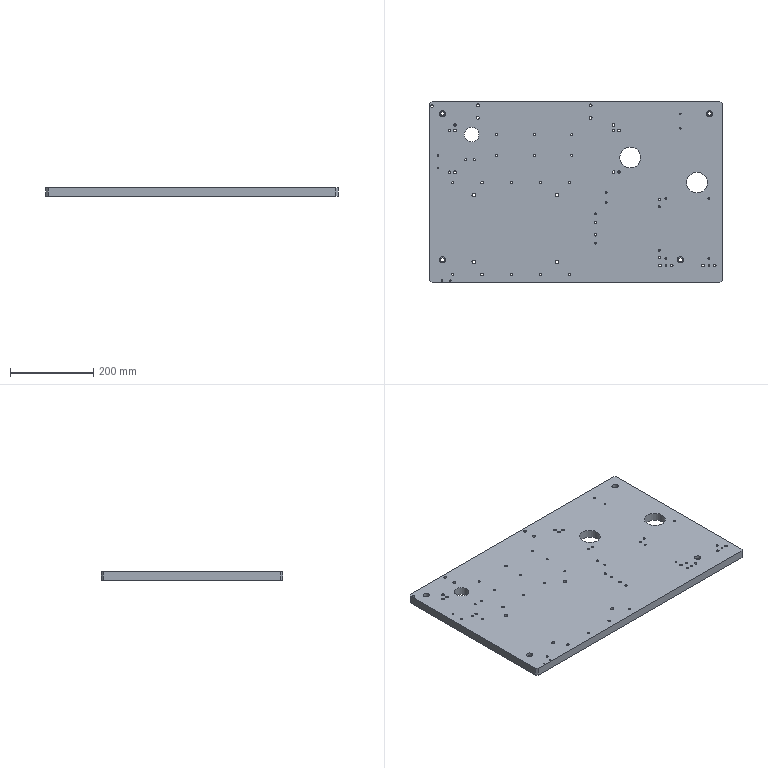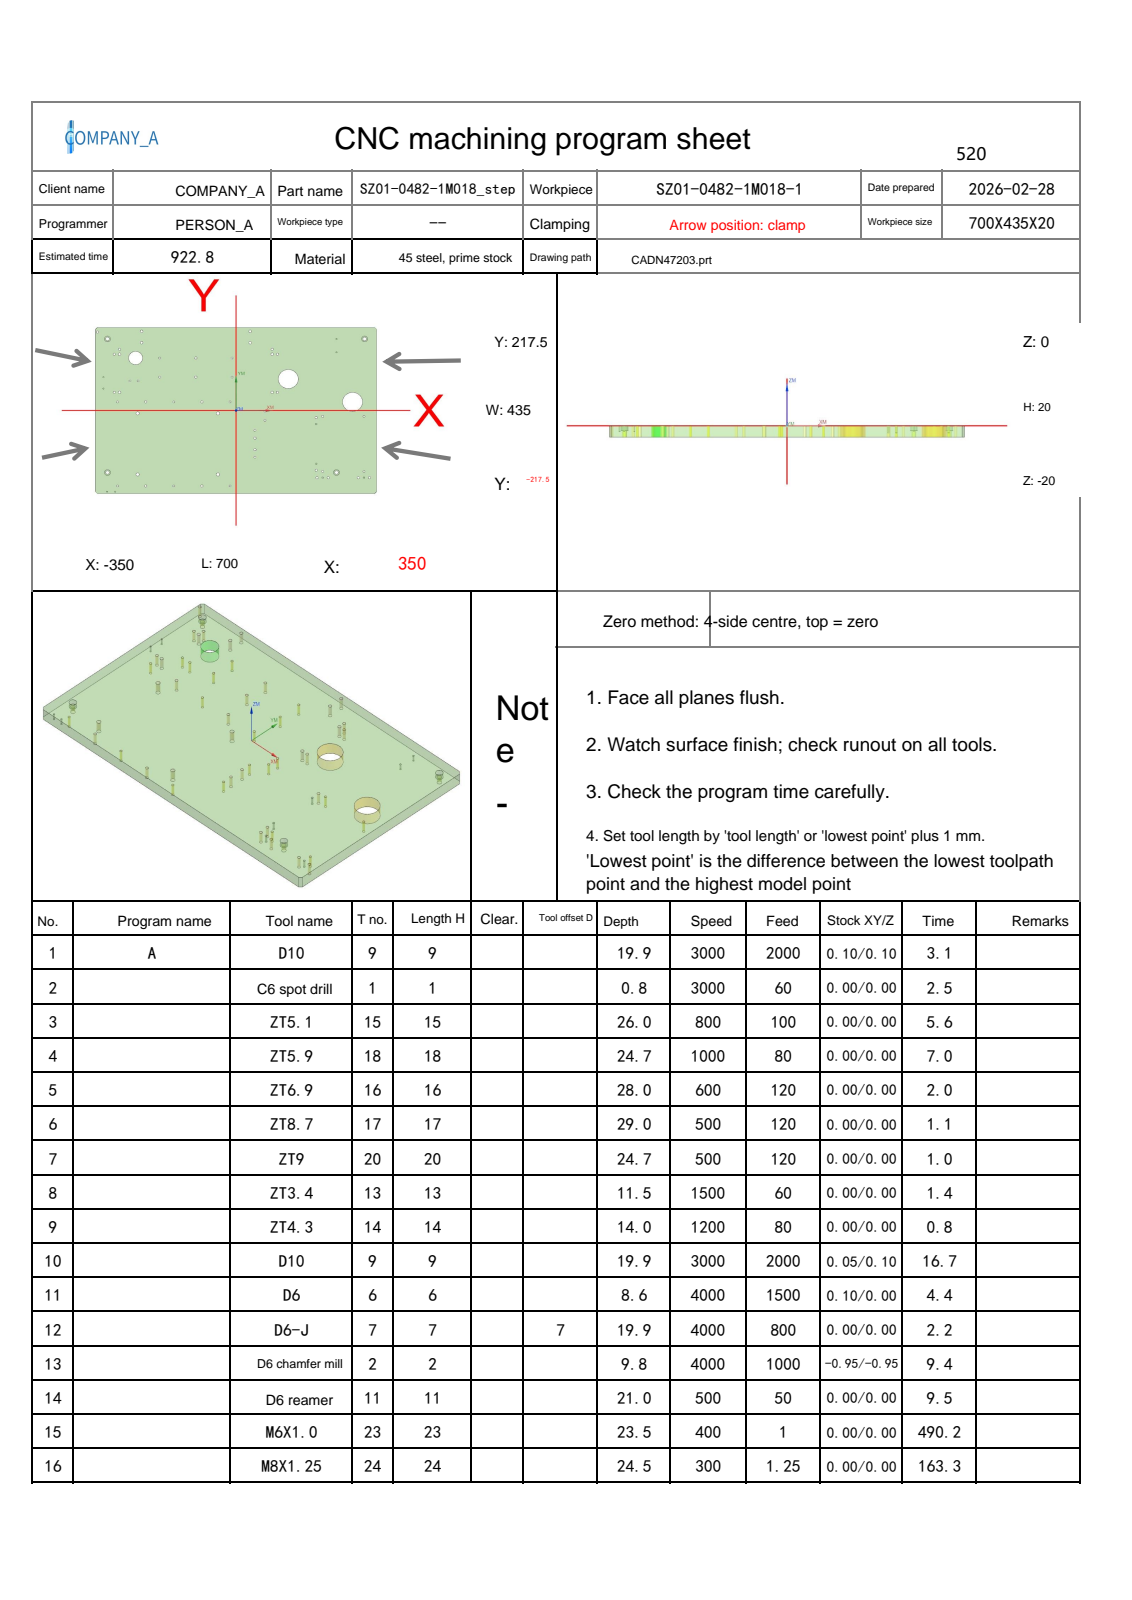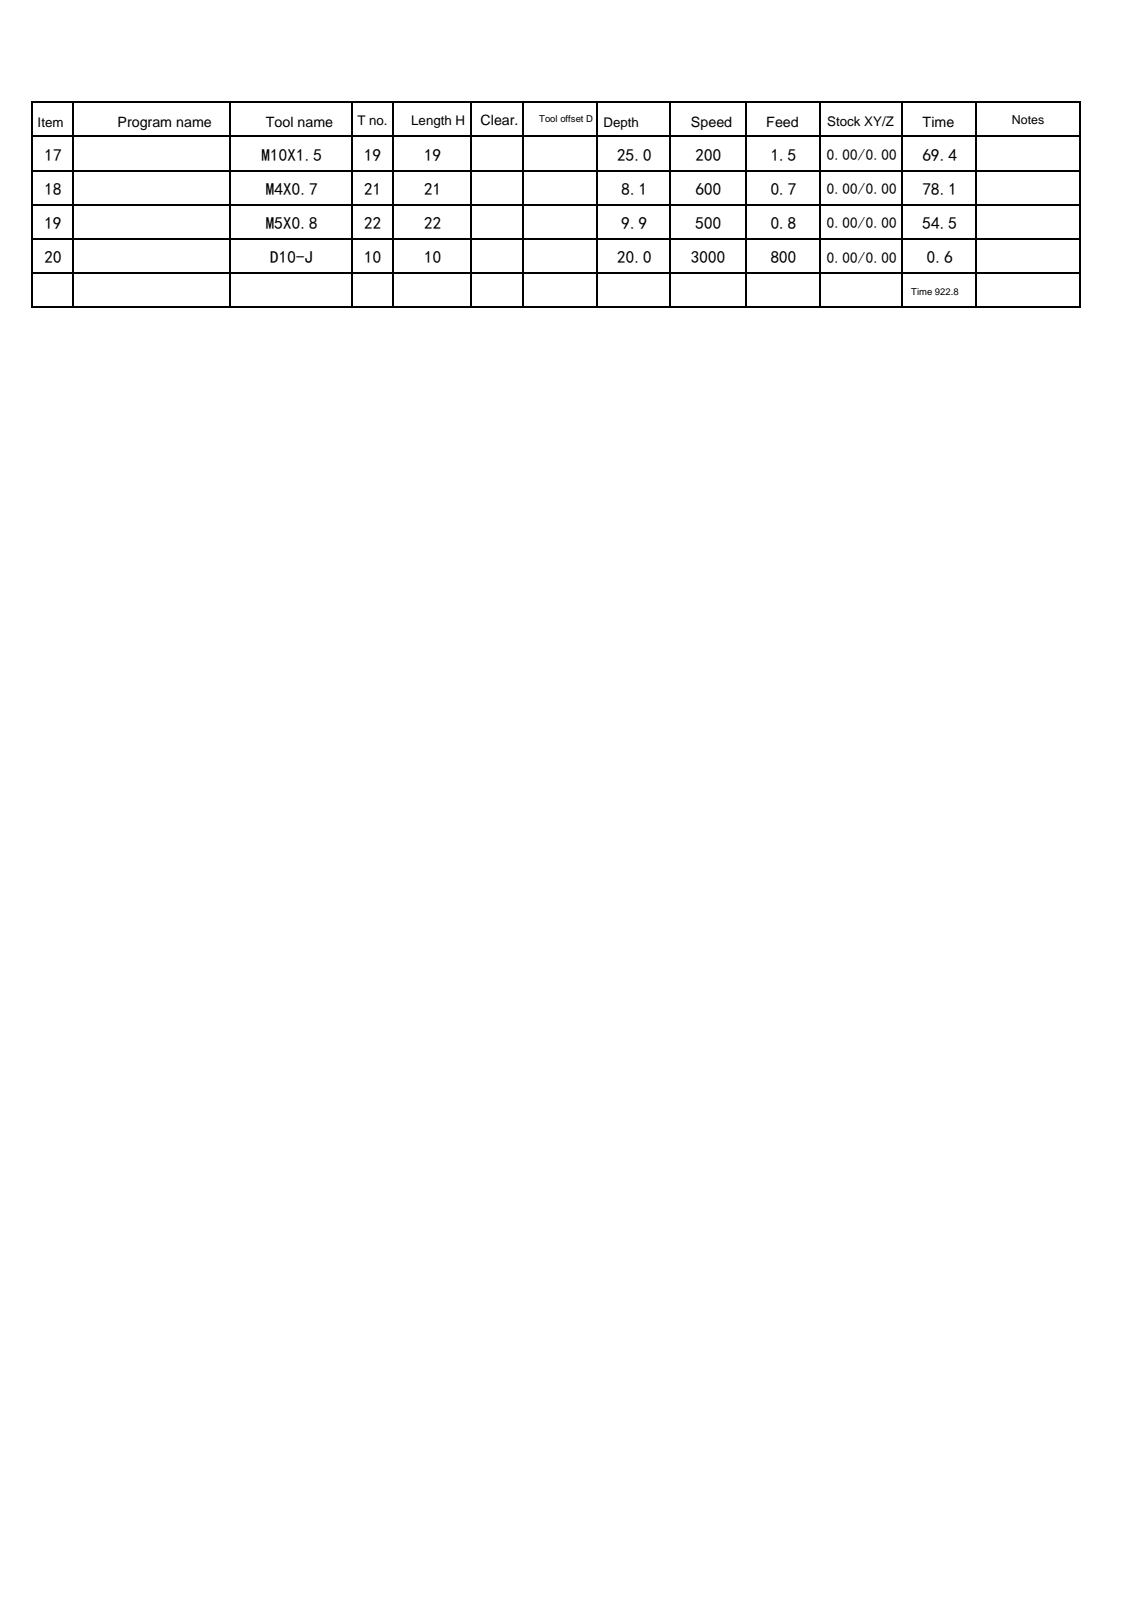NC program | NX | posted by the shop | part box 700 x 435 x 20 mm
Lines 2453 to 3078 of 5271:
N11 T06 M06
(D6  D=6. R=0. H=06 ce=0.10 di=0.00)
G00 G90 G54 X250. Y-162.5 M03 S4000
G43 H06 Z50.
M08
Z.5
G03 X251.1 Y-163.6 I1.1 J0.0 F1500.
X252.2 Y-162.5 I0.0 J1.1
X252.2 Y-162.5 Z.25 I-2.2 J0.0
X252.2 Y-162.5 Z0.0 I-2.2 J0.0
X252.2 Y-162.5 Z-.25 I-2.2 J0.0
X252.2 Y-162.5 Z-.5 I-2.2 J0.0
X252.2 Y-162.5 Z-.75 I-2.2 J0.0
X252.2 Y-162.5 Z-1. I-2.2 J0.0
X252.2 Y-162.5 Z-1.25 I-2.2 J0.0
X252.2 Y-162.5 Z-1.5 I-2.2 J0.0
X252.2 Y-162.5 Z-1.75 I-2.2 J0.0
X252.2 Y-162.5 Z-2. I-2.2 J0.0
X252.2 Y-162.5 Z-2.25 I-2.2 J0.0
X252.2 Y-162.5 Z-2.5 I-2.2 J0.0
X252.2 Y-162.5 Z-2.75 I-2.2 J0.0
X252.2 Y-162.5 Z-3. I-2.2 J0.0
X252.2 Y-162.5 Z-3.25 I-2.2 J0.0
X252.2 Y-162.5 Z-3.5 I-2.2 J0.0
X252.2 Y-162.5 Z-3.75 I-2.2 J0.0
X252.2 Y-162.5 Z-4. I-2.2 J0.0
X252.2 Y-162.5 Z-4.25 I-2.2 J0.0
X252.2 Y-162.5 Z-4.5 I-2.2 J0.0
X252.2 Y-162.5 Z-4.75 I-2.2 J0.0
X252.2 Y-162.5 Z-5. I-2.2 J0.0
X252.2 Y-162.5 Z-5.25 I-2.2 J0.0
X252.2 Y-162.5 Z-5.5 I-2.2 J0.0
X252.2 Y-162.5 Z-5.75 I-2.2 J0.0
X252.2 Y-162.5 Z-6. I-2.2 J0.0
X252.2 Y-162.5 Z-6.25 I-2.2 J0.0
X252.2 Y-162.5 Z-6.5 I-2.2 J0.0
X252.2 Y-162.5 Z-6.75 I-2.2 J0.0
X252.2 Y-162.5 Z-7. I-2.2 J0.0
X252.2 Y-162.5 Z-7.25 I-2.2 J0.0
X252.2 Y-162.5 Z-7.5 I-2.2 J0.0
X252.2 Y-162.5 Z-7.75 I-2.2 J0.0
X252.2 Y-162.5 Z-8. I-2.2 J0.0
X252.2 Y-162.5 Z-8.25 I-2.2 J0.0
X252.2 Y-162.5 Z-8.5 I-2.2 J0.0
X248.22 Y-161.207 Z-8.6 I-2.2 J0.0
X247.8 Y-162.5 I1.78 J-1.293
X250. Y-164.7 I2.2 J0.0
X252.2 Y-162.5 I0.0 J2.2
X250. Y-160.3 I-2.2 J0.0
X248.22 Y-161.207 I0.0 J-2.2
X248.01 Y-161.853 I.89 J-.647
X249.11 Y-162.953 I1.1 J0.0
X250. Y-162.5 I0.0 J1.1
G00 Z.5
G03 X252.2 Y-164.7 I2.2 J0.0
X254.4 Y-162.5 I0.0 J2.2
X254.4 Y-162.5 Z.25 I-4.4 J0.0
X254.4 Y-162.5 Z0.0 I-4.4 J0.0
X254.4 Y-162.5 Z-.25 I-4.4 J0.0
X254.4 Y-162.5 Z-.5 I-4.4 J0.0
X254.4 Y-162.5 Z-.75 I-4.4 J0.0
X254.4 Y-162.5 Z-1. I-4.4 J0.0
X254.4 Y-162.5 Z-1.25 I-4.4 J0.0
X254.4 Y-162.5 Z-1.5 I-4.4 J0.0
X254.4 Y-162.5 Z-1.75 I-4.4 J0.0
X254.4 Y-162.5 Z-2. I-4.4 J0.0
X254.4 Y-162.5 Z-2.25 I-4.4 J0.0
X254.4 Y-162.5 Z-2.5 I-4.4 J0.0
X254.4 Y-162.5 Z-2.75 I-4.4 J0.0
X254.4 Y-162.5 Z-3. I-4.4 J0.0
X254.4 Y-162.5 Z-3.25 I-4.4 J0.0
X254.4 Y-162.5 Z-3.5 I-4.4 J0.0
X254.4 Y-162.5 Z-3.75 I-4.4 J0.0
X254.4 Y-162.5 Z-4. I-4.4 J0.0
X254.4 Y-162.5 Z-4.25 I-4.4 J0.0
X254.4 Y-162.5 Z-4.5 I-4.4 J0.0
X254.4 Y-162.5 Z-4.75 I-4.4 J0.0
X254.4 Y-162.5 Z-5. I-4.4 J0.0
X254.4 Y-162.5 Z-5.25 I-4.4 J0.0
X254.4 Y-162.5 Z-5.5 I-4.4 J0.0
X254.4 Y-162.5 Z-5.75 I-4.4 J0.0
X254.4 Y-162.5 Z-6. I-4.4 J0.0
X254.4 Y-162.5 Z-6.25 I-4.4 J0.0
X254.4 Y-162.5 Z-6.5 I-4.4 J0.0
X254.4 Y-162.5 Z-6.75 I-4.4 J0.0
X254.4 Y-162.5 Z-7. I-4.4 J0.0
X254.4 Y-162.5 Z-7.25 I-4.4 J0.0
X254.4 Y-162.5 Z-7.5 I-4.4 J0.0
X254.4 Y-162.5 Z-7.75 I-4.4 J0.0
X254.4 Y-162.5 Z-8. I-4.4 J0.0
X254.4 Y-162.5 Z-8.25 I-4.4 J0.0
X254.4 Y-162.5 Z-8.5 I-4.4 J0.0
X246.44 Y-159.914 Z-8.6 I-4.4 J0.0
X245.6 Y-162.5 I3.56 J-2.586
X250. Y-166.9 I4.4 J0.0
X254.4 Y-162.5 I0.0 J4.4
X250. Y-158.1 I-4.4 J0.0
X246.44 Y-159.914 I0.0 J-4.4
X246.02 Y-161.207 I1.78 J-1.293
X248.22 Y-163.407 I2.2 J0.0
X250. Y-162.5 I0.0 J2.2
G00 Z50.
X320. Y187.5
Z.5
G03 X321.1 Y186.4 I1.1 J0.0
X322.2 Y187.5 I0.0 J1.1
X322.2 Y187.5 Z.25 I-2.2 J0.0
X322.2 Y187.5 Z0.0 I-2.2 J0.0
X322.2 Y187.5 Z-.25 I-2.2 J0.0
X322.2 Y187.5 Z-.5 I-2.2 J0.0
X322.2 Y187.5 Z-.75 I-2.2 J0.0
X322.2 Y187.5 Z-1. I-2.2 J0.0
X322.2 Y187.5 Z-1.25 I-2.2 J0.0
X322.2 Y187.5 Z-1.5 I-2.2 J0.0
X322.2 Y187.5 Z-1.75 I-2.2 J0.0
X322.2 Y187.5 Z-2. I-2.2 J0.0
X322.2 Y187.5 Z-2.25 I-2.2 J0.0
X322.2 Y187.5 Z-2.5 I-2.2 J0.0
X322.2 Y187.5 Z-2.75 I-2.2 J0.0
X322.2 Y187.5 Z-3. I-2.2 J0.0
X322.2 Y187.5 Z-3.25 I-2.2 J0.0
X322.2 Y187.5 Z-3.5 I-2.2 J0.0
X322.2 Y187.5 Z-3.75 I-2.2 J0.0
X322.2 Y187.5 Z-4. I-2.2 J0.0
X322.2 Y187.5 Z-4.25 I-2.2 J0.0
X322.2 Y187.5 Z-4.5 I-2.2 J0.0
X322.2 Y187.5 Z-4.75 I-2.2 J0.0
X322.2 Y187.5 Z-5. I-2.2 J0.0
X322.2 Y187.5 Z-5.25 I-2.2 J0.0
X322.2 Y187.5 Z-5.5 I-2.2 J0.0
X322.2 Y187.5 Z-5.75 I-2.2 J0.0
X322.2 Y187.5 Z-6. I-2.2 J0.0
X322.2 Y187.5 Z-6.25 I-2.2 J0.0
X322.2 Y187.5 Z-6.5 I-2.2 J0.0
X322.2 Y187.5 Z-6.75 I-2.2 J0.0
X322.2 Y187.5 Z-7. I-2.2 J0.0
X322.2 Y187.5 Z-7.25 I-2.2 J0.0
X322.2 Y187.5 Z-7.5 I-2.2 J0.0
X322.2 Y187.5 Z-7.75 I-2.2 J0.0
X322.2 Y187.5 Z-8. I-2.2 J0.0
X322.2 Y187.5 Z-8.25 I-2.2 J0.0
X322.2 Y187.5 Z-8.5 I-2.2 J0.0
X318.22 Y188.793 Z-8.6 I-2.2 J0.0
X317.8 Y187.5 I1.78 J-1.293
X320. Y185.3 I2.2 J0.0
X322.2 Y187.5 I0.0 J2.2
X320. Y189.7 I-2.2 J0.0
X318.22 Y188.793 I0.0 J-2.2
X318.01 Y188.147 I.89 J-.647
X319.11 Y187.047 I1.1 J0.0
X320. Y187.5 I0.0 J1.1
G00 Z.5
G03 X322.2 Y185.3 I2.2 J0.0
X324.4 Y187.5 I0.0 J2.2
X324.4 Y187.5 Z.25 I-4.4 J0.0
X324.4 Y187.5 Z0.0 I-4.4 J0.0
X324.4 Y187.5 Z-.25 I-4.4 J0.0
X324.4 Y187.5 Z-.5 I-4.4 J0.0
X324.4 Y187.5 Z-.75 I-4.4 J0.0
X324.4 Y187.5 Z-1. I-4.4 J0.0
X324.4 Y187.5 Z-1.25 I-4.4 J0.0
X324.4 Y187.5 Z-1.5 I-4.4 J0.0
X324.4 Y187.5 Z-1.75 I-4.4 J0.0
X324.4 Y187.5 Z-2. I-4.4 J0.0
X324.4 Y187.5 Z-2.25 I-4.4 J0.0
X324.4 Y187.5 Z-2.5 I-4.4 J0.0
X324.4 Y187.5 Z-2.75 I-4.4 J0.0
X324.4 Y187.5 Z-3. I-4.4 J0.0
X324.4 Y187.5 Z-3.25 I-4.4 J0.0
X324.4 Y187.5 Z-3.5 I-4.4 J0.0
X324.4 Y187.5 Z-3.75 I-4.4 J0.0
X324.4 Y187.5 Z-4. I-4.4 J0.0
X324.4 Y187.5 Z-4.25 I-4.4 J0.0
X324.4 Y187.5 Z-4.5 I-4.4 J0.0
X324.4 Y187.5 Z-4.75 I-4.4 J0.0
X324.4 Y187.5 Z-5. I-4.4 J0.0
X324.4 Y187.5 Z-5.25 I-4.4 J0.0
X324.4 Y187.5 Z-5.5 I-4.4 J0.0
X324.4 Y187.5 Z-5.75 I-4.4 J0.0
X324.4 Y187.5 Z-6. I-4.4 J0.0
X324.4 Y187.5 Z-6.25 I-4.4 J0.0
X324.4 Y187.5 Z-6.5 I-4.4 J0.0
X324.4 Y187.5 Z-6.75 I-4.4 J0.0
X324.4 Y187.5 Z-7. I-4.4 J0.0
X324.4 Y187.5 Z-7.25 I-4.4 J0.0
X324.4 Y187.5 Z-7.5 I-4.4 J0.0
X324.4 Y187.5 Z-7.75 I-4.4 J0.0
X324.4 Y187.5 Z-8. I-4.4 J0.0
X324.4 Y187.5 Z-8.25 I-4.4 J0.0
X324.4 Y187.5 Z-8.5 I-4.4 J0.0
X316.44 Y190.086 Z-8.6 I-4.4 J0.0
X315.6 Y187.5 I3.56 J-2.586
X320. Y183.1 I4.4 J0.0
X324.4 Y187.5 I0.0 J4.4
X320. Y191.9 I-4.4 J0.0
X316.44 Y190.086 I0.0 J-4.4
X316.02 Y188.793 I1.78 J-1.293
X318.22 Y186.593 I2.2 J0.0
X320. Y187.5 I0.0 J2.2
G00 Z50.
X-320.
Z.5
G03 X-318.9 Y186.4 I1.1 J0.0
X-317.8 Y187.5 I0.0 J1.1
X-317.8 Y187.5 Z.25 I-2.2 J0.0
X-317.8 Y187.5 Z0.0 I-2.2 J0.0
X-317.8 Y187.5 Z-.25 I-2.2 J0.0
X-317.8 Y187.5 Z-.5 I-2.2 J0.0
X-317.8 Y187.5 Z-.75 I-2.2 J0.0
X-317.8 Y187.5 Z-1. I-2.2 J0.0
X-317.8 Y187.5 Z-1.25 I-2.2 J0.0
X-317.8 Y187.5 Z-1.5 I-2.2 J0.0
X-317.8 Y187.5 Z-1.75 I-2.2 J0.0
X-317.8 Y187.5 Z-2. I-2.2 J0.0
X-317.8 Y187.5 Z-2.25 I-2.2 J0.0
X-317.8 Y187.5 Z-2.5 I-2.2 J0.0
X-317.8 Y187.5 Z-2.75 I-2.2 J0.0
X-317.8 Y187.5 Z-3. I-2.2 J0.0
X-317.8 Y187.5 Z-3.25 I-2.2 J0.0
X-317.8 Y187.5 Z-3.5 I-2.2 J0.0
X-317.8 Y187.5 Z-3.75 I-2.2 J0.0
X-317.8 Y187.5 Z-4. I-2.2 J0.0
X-317.8 Y187.5 Z-4.25 I-2.2 J0.0
X-317.8 Y187.5 Z-4.5 I-2.2 J0.0
X-317.8 Y187.5 Z-4.75 I-2.2 J0.0
X-317.8 Y187.5 Z-5. I-2.2 J0.0
X-317.8 Y187.5 Z-5.25 I-2.2 J0.0
X-317.8 Y187.5 Z-5.5 I-2.2 J0.0
X-317.8 Y187.5 Z-5.75 I-2.2 J0.0
X-317.8 Y187.5 Z-6. I-2.2 J0.0
X-317.8 Y187.5 Z-6.25 I-2.2 J0.0
X-317.8 Y187.5 Z-6.5 I-2.2 J0.0
X-317.8 Y187.5 Z-6.75 I-2.2 J0.0
X-317.8 Y187.5 Z-7. I-2.2 J0.0
X-317.8 Y187.5 Z-7.25 I-2.2 J0.0
X-317.8 Y187.5 Z-7.5 I-2.2 J0.0
X-317.8 Y187.5 Z-7.75 I-2.2 J0.0
X-317.8 Y187.5 Z-8. I-2.2 J0.0
X-317.8 Y187.5 Z-8.25 I-2.2 J0.0
X-317.8 Y187.5 Z-8.5 I-2.2 J0.0
X-321.78 Y188.793 Z-8.6 I-2.2 J0.0
X-322.2 Y187.5 I1.78 J-1.293
X-320. Y185.3 I2.2 J0.0
X-317.8 Y187.5 I0.0 J2.2
X-320. Y189.7 I-2.2 J0.0
X-321.78 Y188.793 I0.0 J-2.2
X-321.99 Y188.147 I.89 J-.647
X-320.89 Y187.047 I1.1 J0.0
X-320. Y187.5 I0.0 J1.1
G00 Z.5
G03 X-317.8 Y185.3 I2.2 J0.0
X-315.6 Y187.5 I0.0 J2.2
X-315.6 Y187.5 Z.25 I-4.4 J0.0
X-315.6 Y187.5 Z0.0 I-4.4 J0.0
X-315.6 Y187.5 Z-.25 I-4.4 J0.0
X-315.6 Y187.5 Z-.5 I-4.4 J0.0
X-315.6 Y187.5 Z-.75 I-4.4 J0.0
X-315.6 Y187.5 Z-1. I-4.4 J0.0
X-315.6 Y187.5 Z-1.25 I-4.4 J0.0
X-315.6 Y187.5 Z-1.5 I-4.4 J0.0
X-315.6 Y187.5 Z-1.75 I-4.4 J0.0
X-315.6 Y187.5 Z-2. I-4.4 J0.0
X-315.6 Y187.5 Z-2.25 I-4.4 J0.0
X-315.6 Y187.5 Z-2.5 I-4.4 J0.0
X-315.6 Y187.5 Z-2.75 I-4.4 J0.0
X-315.6 Y187.5 Z-3. I-4.4 J0.0
X-315.6 Y187.5 Z-3.25 I-4.4 J0.0
X-315.6 Y187.5 Z-3.5 I-4.4 J0.0
X-315.6 Y187.5 Z-3.75 I-4.4 J0.0
X-315.6 Y187.5 Z-4. I-4.4 J0.0
X-315.6 Y187.5 Z-4.25 I-4.4 J0.0
X-315.6 Y187.5 Z-4.5 I-4.4 J0.0
X-315.6 Y187.5 Z-4.75 I-4.4 J0.0
X-315.6 Y187.5 Z-5. I-4.4 J0.0
X-315.6 Y187.5 Z-5.25 I-4.4 J0.0
X-315.6 Y187.5 Z-5.5 I-4.4 J0.0
X-315.6 Y187.5 Z-5.75 I-4.4 J0.0
X-315.6 Y187.5 Z-6. I-4.4 J0.0
X-315.6 Y187.5 Z-6.25 I-4.4 J0.0
X-315.6 Y187.5 Z-6.5 I-4.4 J0.0
X-315.6 Y187.5 Z-6.75 I-4.4 J0.0
X-315.6 Y187.5 Z-7. I-4.4 J0.0
X-315.6 Y187.5 Z-7.25 I-4.4 J0.0
X-315.6 Y187.5 Z-7.5 I-4.4 J0.0
X-315.6 Y187.5 Z-7.75 I-4.4 J0.0
X-315.6 Y187.5 Z-8. I-4.4 J0.0
X-315.6 Y187.5 Z-8.25 I-4.4 J0.0
X-315.6 Y187.5 Z-8.5 I-4.4 J0.0
X-323.56 Y190.086 Z-8.6 I-4.4 J0.0
X-324.4 Y187.5 I3.56 J-2.586
X-320. Y183.1 I4.4 J0.0
X-315.6 Y187.5 I0.0 J4.4
X-320. Y191.9 I-4.4 J0.0
X-323.56 Y190.086 I0.0 J-4.4
X-323.98 Y188.793 I1.78 J-1.293
X-321.78 Y186.593 I2.2 J0.0
X-320. Y187.5 I0.0 J2.2
G00 Z50.
Y-162.5
Z.5
G03 X-318.9 Y-163.6 I1.1 J0.0
X-317.8 Y-162.5 I0.0 J1.1
X-317.8 Y-162.5 Z.25 I-2.2 J0.0
X-317.8 Y-162.5 Z0.0 I-2.2 J0.0
X-317.8 Y-162.5 Z-.25 I-2.2 J0.0
X-317.8 Y-162.5 Z-.5 I-2.2 J0.0
X-317.8 Y-162.5 Z-.75 I-2.2 J0.0
X-317.8 Y-162.5 Z-1. I-2.2 J0.0
X-317.8 Y-162.5 Z-1.25 I-2.2 J0.0
X-317.8 Y-162.5 Z-1.5 I-2.2 J0.0
X-317.8 Y-162.5 Z-1.75 I-2.2 J0.0
X-317.8 Y-162.5 Z-2. I-2.2 J0.0
X-317.8 Y-162.5 Z-2.25 I-2.2 J0.0
X-317.8 Y-162.5 Z-2.5 I-2.2 J0.0
X-317.8 Y-162.5 Z-2.75 I-2.2 J0.0
X-317.8 Y-162.5 Z-3. I-2.2 J0.0
X-317.8 Y-162.5 Z-3.25 I-2.2 J0.0
X-317.8 Y-162.5 Z-3.5 I-2.2 J0.0
X-317.8 Y-162.5 Z-3.75 I-2.2 J0.0
X-317.8 Y-162.5 Z-4. I-2.2 J0.0
X-317.8 Y-162.5 Z-4.25 I-2.2 J0.0
X-317.8 Y-162.5 Z-4.5 I-2.2 J0.0
X-317.8 Y-162.5 Z-4.75 I-2.2 J0.0
X-317.8 Y-162.5 Z-5. I-2.2 J0.0
X-317.8 Y-162.5 Z-5.25 I-2.2 J0.0
X-317.8 Y-162.5 Z-5.5 I-2.2 J0.0
X-317.8 Y-162.5 Z-5.75 I-2.2 J0.0
X-317.8 Y-162.5 Z-6. I-2.2 J0.0
X-317.8 Y-162.5 Z-6.25 I-2.2 J0.0
X-317.8 Y-162.5 Z-6.5 I-2.2 J0.0
X-317.8 Y-162.5 Z-6.75 I-2.2 J0.0
X-317.8 Y-162.5 Z-7. I-2.2 J0.0
X-317.8 Y-162.5 Z-7.25 I-2.2 J0.0
X-317.8 Y-162.5 Z-7.5 I-2.2 J0.0
X-317.8 Y-162.5 Z-7.75 I-2.2 J0.0
X-317.8 Y-162.5 Z-8. I-2.2 J0.0
X-317.8 Y-162.5 Z-8.25 I-2.2 J0.0
X-317.8 Y-162.5 Z-8.5 I-2.2 J0.0
X-321.78 Y-161.207 Z-8.6 I-2.2 J0.0
X-322.2 Y-162.5 I1.78 J-1.293
X-320. Y-164.7 I2.2 J0.0
X-317.8 Y-162.5 I0.0 J2.2
X-320. Y-160.3 I-2.2 J0.0
X-321.78 Y-161.207 I0.0 J-2.2
X-321.99 Y-161.853 I.89 J-.647
X-320.89 Y-162.953 I1.1 J0.0
X-320. Y-162.5 I0.0 J1.1
G00 Z.5
G03 X-317.8 Y-164.7 I2.2 J0.0
X-315.6 Y-162.5 I0.0 J2.2
X-315.6 Y-162.5 Z.25 I-4.4 J0.0
X-315.6 Y-162.5 Z0.0 I-4.4 J0.0
X-315.6 Y-162.5 Z-.25 I-4.4 J0.0
X-315.6 Y-162.5 Z-.5 I-4.4 J0.0
X-315.6 Y-162.5 Z-.75 I-4.4 J0.0
X-315.6 Y-162.5 Z-1. I-4.4 J0.0
X-315.6 Y-162.5 Z-1.25 I-4.4 J0.0
X-315.6 Y-162.5 Z-1.5 I-4.4 J0.0
X-315.6 Y-162.5 Z-1.75 I-4.4 J0.0
X-315.6 Y-162.5 Z-2. I-4.4 J0.0
X-315.6 Y-162.5 Z-2.25 I-4.4 J0.0
X-315.6 Y-162.5 Z-2.5 I-4.4 J0.0
X-315.6 Y-162.5 Z-2.75 I-4.4 J0.0
X-315.6 Y-162.5 Z-3. I-4.4 J0.0
X-315.6 Y-162.5 Z-3.25 I-4.4 J0.0
X-315.6 Y-162.5 Z-3.5 I-4.4 J0.0
X-315.6 Y-162.5 Z-3.75 I-4.4 J0.0
X-315.6 Y-162.5 Z-4. I-4.4 J0.0
X-315.6 Y-162.5 Z-4.25 I-4.4 J0.0
X-315.6 Y-162.5 Z-4.5 I-4.4 J0.0
X-315.6 Y-162.5 Z-4.75 I-4.4 J0.0
X-315.6 Y-162.5 Z-5. I-4.4 J0.0
X-315.6 Y-162.5 Z-5.25 I-4.4 J0.0
X-315.6 Y-162.5 Z-5.5 I-4.4 J0.0
X-315.6 Y-162.5 Z-5.75 I-4.4 J0.0
X-315.6 Y-162.5 Z-6. I-4.4 J0.0
X-315.6 Y-162.5 Z-6.25 I-4.4 J0.0
X-315.6 Y-162.5 Z-6.5 I-4.4 J0.0
X-315.6 Y-162.5 Z-6.75 I-4.4 J0.0
X-315.6 Y-162.5 Z-7. I-4.4 J0.0
X-315.6 Y-162.5 Z-7.25 I-4.4 J0.0
X-315.6 Y-162.5 Z-7.5 I-4.4 J0.0
X-315.6 Y-162.5 Z-7.75 I-4.4 J0.0
X-315.6 Y-162.5 Z-8. I-4.4 J0.0
X-315.6 Y-162.5 Z-8.25 I-4.4 J0.0
X-315.6 Y-162.5 Z-8.5 I-4.4 J0.0
X-323.56 Y-159.914 Z-8.6 I-4.4 J0.0
X-324.4 Y-162.5 I3.56 J-2.586
X-320. Y-166.9 I4.4 J0.0
X-315.6 Y-162.5 I0.0 J4.4
X-320. Y-158.1 I-4.4 J0.0
X-323.56 Y-159.914 I0.0 J-4.4
X-323.98 Y-161.207 I1.78 J-1.293
X-321.78 Y-163.407 I2.2 J0.0
X-320. Y-162.5 I0.0 J2.2
G00 Z50.
G91 G28 Z0.0
M05
M09
G91 G28 Z0.0
M01
N12 T07 M06
(D6-J  D=6. R=0. H=07 ce=0.00 di=0.00)
G00 G90 G54 X250. Y-162.5 M03 S4000
G43 H07 Z50.
M08
Z.5
G41 D07
G01 X250.794 Y-163.653 F800.
G03 X252.468 Y-164.532 I1.674 J1.153
X254.5 Y-162.5 I0.0 J2.032
X254.5 Y-162.5 Z-4.5 I-4.5 J0.0
X251.916 Y-166.572 Z-8.6 I-4.5 J0.0
X254.5 Y-162.5 I-1.916 J4.072
X250. Y-158. I-4.5 J0.0
X245.5 Y-162.5 I0.0 J-4.5
X250. Y-167. I4.5 J0.0
X251.916 Y-166.572 I0.0 J4.5
X253.083 Y-164.733 I-.865 J1.839
X251.381 Y-162.728 I-2.032 J0.0
G01 G40 X250. Y-162.5
G00 Z50.
X320. Y187.5
Z.5
G41 D07
G01 X320.794 Y186.347
G03 X322.468 Y185.468 I1.674 J1.153
X324.5 Y187.5 I0.0 J2.032
X324.5 Y187.5 Z-4.5 I-4.5 J0.0
X321.916 Y183.428 Z-8.6 I-4.5 J0.0
X324.5 Y187.5 I-1.916 J4.072
X320. Y192. I-4.5 J0.0
X315.5 Y187.5 I0.0 J-4.5
X320. Y183. I4.5 J0.0
X321.916 Y183.428 I0.0 J4.5
X323.083 Y185.267 I-.865 J1.839
X321.381 Y187.272 I-2.032 J0.0
G01 G40 X320. Y187.5
G00 Z50.
X-320.
Z.5
G41 D07
G01 X-319.206 Y186.347
G03 X-317.532 Y185.468 I1.674 J1.153
X-315.5 Y187.5 I0.0 J2.032
X-315.5 Y187.5 Z-4.5 I-4.5 J0.0
X-318.084 Y183.428 Z-8.6 I-4.5 J0.0
X-315.5 Y187.5 I-1.916 J4.072
X-320. Y192. I-4.5 J0.0
X-324.5 Y187.5 I0.0 J-4.5
X-320. Y183. I4.5 J0.0
X-318.084 Y183.428 I0.0 J4.5
X-316.917 Y185.267 I-.865 J1.839
X-318.619 Y187.272 I-2.032 J0.0
G01 G40 X-320. Y187.5
G00 Z50.
Y-162.5
Z.5
G41 D07
G01 X-319.206 Y-163.653
G03 X-317.532 Y-164.532 I1.674 J1.153
X-315.5 Y-162.5 I0.0 J2.032
X-315.5 Y-162.5 Z-4.5 I-4.5 J0.0
X-318.084 Y-166.572 Z-8.6 I-4.5 J0.0
X-315.5 Y-162.5 I-1.916 J4.072
X-320. Y-158. I-4.5 J0.0
X-324.5 Y-162.5 I0.0 J-4.5
X-320. Y-167. I4.5 J0.0
X-318.084 Y-166.572 I0.0 J4.5
X-316.917 Y-164.733 I-.865 J1.839
X-318.619 Y-162.728 I-2.032 J0.0
G01 G40 X-320. Y-162.5
G00 Z50.
G00 G90 X-249.1 Y150.87 M03 S3500
Z10.
Z-5.133
G01 Z-6.633 F800.
G41 D07
Y151.1
G03 X-250. Y152. I-.9 J0.0
X-264.5 Y137.5 I0.0 J-14.5
X-250. Y123. I14.5 J0.0
X-235.5 Y137.5 I0.0 J14.5
X-250. Y152. I-14.5 J0.0
X-250.4 Y151.994 I0.0 J-14.5
X-251.275 Y151.095 I.025 J-.9
G01 Y151.07
X-251.274 Y151.04
G40 X-251.268 Y150.84
Z-5.133
G00 X-249.1 Y150.87
Z-11.767
G01 Z-13.267
G41 D07
Y151.1
G03 X-250. Y152. I-.9 J0.0
X-264.5 Y137.5 I0.0 J-14.5
X-250. Y123. I14.5 J0.0
X-235.5 Y137.5 I0.0 J14.5
X-250. Y152. I-14.5 J0.0
X-250.4 Y151.994 I0.0 J-14.5
X-251.275 Y151.095 I.025 J-.9
G01 Y151.07
X-251.274 Y151.04
G40 X-251.268 Y150.84
Z-11.767
G00 X-249.1 Y150.87
Z-18.4
G01 Z-19.9
G41 D07
Y151.1
G03 X-250. Y152. I-.9 J0.0
X-264.5 Y137.5 I0.0 J-14.5
X-250. Y123. I14.5 J0.0
X-235.5 Y137.5 I0.0 J14.5
X-250. Y152. I-14.5 J0.0
X-250.4 Y151.994 I0.0 J-14.5
X-251.275 Y151.095 I.025 J-.9
G01 Y151.07
X-251.274 Y151.04
G40 X-251.268 Y150.84
Z-18.4
G00 Z10.
X130.9 Y103.381
Z-5.133
G01 Z-6.633
G41 D07
Y103.6
G03 X130. Y104.5 I-.9 J0.0
X108. Y82.5 I0.0 J-22.
X130. Y60.5 I22. J0.0
X152. Y82.5 I0.0 J22.
X130. Y104.5 I-22. J0.0
X129.6 Y104.496 I0.0 J-22.
X128.716 Y103.597 I.016 J-.9
G01 X128.717 Y103.58
Y103.561
G40 X128.721 Y103.361
Z-5.133
G00 X130.9 Y103.381
Z-11.767
G01 Z-13.267
G41 D07
Y103.6
G03 X130. Y104.5 I-.9 J0.0
X108. Y82.5 I0.0 J-22.
X130. Y60.5 I22. J0.0
X152. Y82.5 I0.0 J22.
X130. Y104.5 I-22. J0.0
X129.6 Y104.496 I0.0 J-22.
X128.716 Y103.597 I.016 J-.9
G01 X128.717 Y103.58
Y103.561
G40 X128.721 Y103.361
Z-11.767
G00 X130.9 Y103.381
Z-18.4
G01 Z-19.9
G41 D07
Y103.6
G03 X130. Y104.5 I-.9 J0.0
X108. Y82.5 I0.0 J-22.
X130. Y60.5 I22. J0.0
X152. Y82.5 I0.0 J22.
X130. Y104.5 I-22. J0.0
X129.6 Y104.496 I0.0 J-22.
X128.716 Y103.597 I.016 J-.9
G01 X128.717 Y103.58
Y103.561
G40 X128.721 Y103.361
Z-18.4
G00 Z10.
X310.881 Y21.6
Z-5.133
G01 Z-6.633
G41 D07
X311.1
G03 X312. Y22.5 I0.0 J.9
X290. Y44.5 I-22. J0.0
X268. Y22.5 I0.0 J-22.
X290. Y.5 I22. J0.0
X312. Y22.5 I0.0 J22.
X311.996 Y22.9 I-22. J0.0
X311.097 Y23.784 I-.9 J-.016
G01 X311.08 Y23.783
X311.061
G40 X310.861 Y23.779
Z-5.133
G00 X310.881 Y21.6
Z-11.767
G01 Z-13.267
G41 D07
X311.1
G03 X312. Y22.5 I0.0 J.9
X290. Y44.5 I-22. J0.0
X268. Y22.5 I0.0 J-22.
X290. Y.5 I22. J0.0
X312. Y22.5 I0.0 J22.
X311.996 Y22.9 I-22. J0.0
X311.097 Y23.784 I-.9 J-.016
G01 X311.08 Y23.783
X311.061
G40 X310.861 Y23.779
Z-11.767
G00 X310.881 Y21.6
Z-18.4
G01 Z-19.9
G41 D07
X311.1
G03 X312. Y22.5 I0.0 J.9
X290. Y44.5 I-22. J0.0
X268. Y22.5 I0.0 J-22.
X290. Y.5 I22. J0.0
X312. Y22.5 I0.0 J22.
X311.996 Y22.9 I-22. J0.0
X311.097 Y23.784 I-.9 J-.016
G01 X311.08 Y23.783
X311.061
G40 X310.861 Y23.779
Z-18.4
G00 Z10.
G91 G28 Z0.0
M05
M09
G91 G28 Z0.0
M01